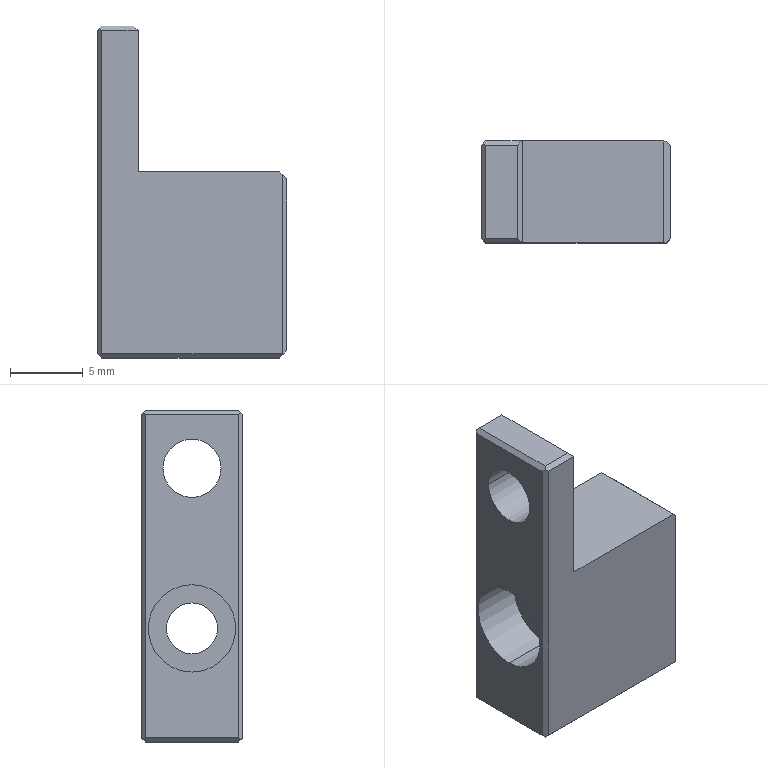Part | NX | 1 solid | 28 faces | box 13 x 7 x 22.8 mm | volume 1128 mm3 | plane 22 | cylinder 6 | commonest cylinder face diameters 3.5 x2 4 x2 6 x2
STEP:
#1=CARTESIAN_POINT('',(2192.3,158.2,-92.));
#2=VERTEX_POINT('',#1);
#3=CARTESIAN_POINT('',(2192.3,151.8,-92.));
#4=VERTEX_POINT('',#3);
#5=CARTESIAN_POINT('',(2192.3,155.,-92.));
#6=DIRECTION('',(0.,-1.,0.));
#7=VECTOR('',#6,1000.);
#8=LINE('',#5,#7);
#9=EDGE_CURVE('',#2,#4,#8,.T.);
#10=ORIENTED_EDGE('',*,*,#9,.T.);
#11=CARTESIAN_POINT('',(2194.5,151.8,-92.));
#12=VERTEX_POINT('',#11);
#13=CARTESIAN_POINT('',(2193.4,151.8,-92.));
#14=DIRECTION('',(-1.,0.,0.));
#15=VECTOR('',#14,1000.);
#16=LINE('',#13,#15);
#17=EDGE_CURVE('',#12,#4,#16,.T.);
#18=ORIENTED_EDGE('',*,*,#17,.F.);
#19=CARTESIAN_POINT('',(2194.5,158.2,-92.));
#20=VERTEX_POINT('',#19);
#21=CARTESIAN_POINT('',(2194.5,155.,-92.));
#22=DIRECTION('',(0.,1.,0.));
#23=VECTOR('',#22,1000.);
#24=LINE('',#21,#23);
#25=EDGE_CURVE('',#12,#20,#24,.T.);
#26=ORIENTED_EDGE('',*,*,#25,.T.);
#27=CARTESIAN_POINT('',(2193.4,158.2,-92.));
#28=DIRECTION('',(-1.,0.,0.));
#29=VECTOR('',#28,1000.);
#30=LINE('',#27,#29);
#31=EDGE_CURVE('',#20,#2,#30,.T.);
#32=ORIENTED_EDGE('',*,*,#31,.T.);
#33=EDGE_LOOP('',(#10,#18,#26,#32));
#34=FACE_BOUND('',#33,.T.);
#35=CARTESIAN_POINT('',(2192.,158.5,-92.));
#36=DIRECTION('',(0.,0.,1.));
#37=DIRECTION('',(1.,0.,0.));
#38=AXIS2_PLACEMENT_3D('',#35,#36,#37);
#39=PLANE('',#38);
#40=ADVANCED_FACE('',(#34),#39,.T.);
#41=CARTESIAN_POINT('',(2192.,158.2,-114.5));
#42=VERTEX_POINT('',#41);
#43=CARTESIAN_POINT('',(2192.,151.8,-114.5));
#44=VERTEX_POINT('',#43);
#45=CARTESIAN_POINT('',(2192.,155.,-114.5));
#46=DIRECTION('',(0.,-1.,0.));
#47=VECTOR('',#46,1000.);
#48=LINE('',#45,#47);
#49=EDGE_CURVE('',#42,#44,#48,.T.);
#50=ORIENTED_EDGE('',*,*,#49,.T.);
#51=CARTESIAN_POINT('',(2192.,151.8,-92.3));
#52=VERTEX_POINT('',#51);
#53=CARTESIAN_POINT('',(2192.,151.8,-102.539));
#54=DIRECTION('',(0.,0.,1.));
#55=VECTOR('',#54,1000.);
#56=LINE('',#53,#55);
#57=EDGE_CURVE('',#44,#52,#56,.T.);
#58=ORIENTED_EDGE('',*,*,#57,.T.);
#59=CARTESIAN_POINT('',(2192.,158.2,-92.3));
#60=VERTEX_POINT('',#59);
#61=CARTESIAN_POINT('',(2192.,155.,-92.3));
#62=DIRECTION('',(0.,-1.,0.));
#63=VECTOR('',#62,1000.);
#64=LINE('',#61,#63);
#65=EDGE_CURVE('',#60,#52,#64,.T.);
#66=ORIENTED_EDGE('',*,*,#65,.F.);
#67=CARTESIAN_POINT('',(2192.,158.2,-102.539));
#68=DIRECTION('',(0.,0.,1.));
#69=VECTOR('',#68,1000.);
#70=LINE('',#67,#69);
#71=EDGE_CURVE('',#42,#60,#70,.T.);
#72=ORIENTED_EDGE('',*,*,#71,.F.);
#73=EDGE_LOOP('',(#50,#58,#66,#72));
#74=FACE_BOUND('',#73,.T.);
#75=CARTESIAN_POINT('',(2192.,153.,-96.));
#76=VERTEX_POINT('',#75);
#77=CARTESIAN_POINT('',(2192.,157.,-96.));
#78=VERTEX_POINT('',#77);
#79=CARTESIAN_POINT('',(2192.,155.,-96.));
#80=DIRECTION('',(1.,0.,0.));
#81=DIRECTION('',(0.,1.,0.));
#82=AXIS2_PLACEMENT_3D('',#79,#80,#81);
#83=CIRCLE('',#82,2.);
#84=EDGE_CURVE('',#76,#78,#83,.T.);
#85=ORIENTED_EDGE('',*,*,#84,.T.);
#86=CARTESIAN_POINT('',(2192.,155.,-96.));
#87=DIRECTION('',(1.,0.,0.));
#88=DIRECTION('',(0.,1.,0.));
#89=AXIS2_PLACEMENT_3D('',#86,#87,#88);
#90=CIRCLE('',#89,2.);
#91=EDGE_CURVE('',#78,#76,#90,.T.);
#92=ORIENTED_EDGE('',*,*,#91,.T.);
#93=EDGE_LOOP('',(#85,#92));
#94=FACE_BOUND('',#93,.T.);
#95=CARTESIAN_POINT('',(2192.,155.,-110.));
#96=VERTEX_POINT('',#95);
#97=CARTESIAN_POINT('',(2192.,155.,-104.));
#98=VERTEX_POINT('',#97);
#99=CARTESIAN_POINT('',(2192.,155.,-107.));
#100=DIRECTION('',(-1.,0.,0.));
#101=DIRECTION('',(0.,0.,-1.));
#102=AXIS2_PLACEMENT_3D('',#99,#100,#101);
#103=CIRCLE('',#102,3.);
#104=EDGE_CURVE('',#96,#98,#103,.T.);
#105=ORIENTED_EDGE('',*,*,#104,.F.);
#106=CARTESIAN_POINT('',(2192.,155.,-107.));
#107=DIRECTION('',(-1.,0.,0.));
#108=DIRECTION('',(0.,0.,-1.));
#109=AXIS2_PLACEMENT_3D('',#106,#107,#108);
#110=CIRCLE('',#109,3.);
#111=EDGE_CURVE('',#98,#96,#110,.T.);
#112=ORIENTED_EDGE('',*,*,#111,.F.);
#113=EDGE_LOOP('',(#105,#112));
#114=FACE_BOUND('',#113,.T.);
#115=CARTESIAN_POINT('',(2192.,158.5,-112.));
#116=DIRECTION('',(-1.,0.,0.));
#117=DIRECTION('',(0.,0.,1.));
#118=AXIS2_PLACEMENT_3D('',#115,#116,#117);
#119=PLANE('',#118);
#120=ADVANCED_FACE('',(#74,#94,#114),#119,.T.);
#121=CARTESIAN_POINT('',(2204.5,151.8,-114.8));
#122=VERTEX_POINT('',#121);
#123=CARTESIAN_POINT('',(2204.5,158.2,-114.8));
#124=VERTEX_POINT('',#123);
#125=CARTESIAN_POINT('',(2204.5,155.,-114.8));
#126=DIRECTION('',(0.,1.,0.));
#127=VECTOR('',#126,1000.);
#128=LINE('',#125,#127);
#129=EDGE_CURVE('',#122,#124,#128,.T.);
#130=ORIENTED_EDGE('',*,*,#129,.F.);
#131=CARTESIAN_POINT('',(2192.3,151.8,-114.8));
#132=VERTEX_POINT('',#131);
#133=CARTESIAN_POINT('',(2198.5,151.8,-114.8));
#134=DIRECTION('',(-1.,0.,0.));
#135=VECTOR('',#134,1000.);
#136=LINE('',#133,#135);
#137=EDGE_CURVE('',#122,#132,#136,.T.);
#138=ORIENTED_EDGE('',*,*,#137,.T.);
#139=CARTESIAN_POINT('',(2192.3,158.2,-114.8));
#140=VERTEX_POINT('',#139);
#141=CARTESIAN_POINT('',(2192.3,155.,-114.8));
#142=DIRECTION('',(0.,-1.,0.));
#143=VECTOR('',#142,1000.);
#144=LINE('',#141,#143);
#145=EDGE_CURVE('',#140,#132,#144,.T.);
#146=ORIENTED_EDGE('',*,*,#145,.F.);
#147=CARTESIAN_POINT('',(2198.5,158.2,-114.8));
#148=DIRECTION('',(-1.,0.,0.));
#149=VECTOR('',#148,1000.);
#150=LINE('',#147,#149);
#151=EDGE_CURVE('',#124,#140,#150,.T.);
#152=ORIENTED_EDGE('',*,*,#151,.F.);
#153=EDGE_LOOP('',(#130,#138,#146,#152));
#154=FACE_BOUND('',#153,.T.);
#155=CARTESIAN_POINT('',(2200.,158.5,-114.8));
#156=DIRECTION('',(0.,0.,-1.));
#157=DIRECTION('',(0.,-1.,0.));
#158=AXIS2_PLACEMENT_3D('',#155,#156,#157);
#159=PLANE('',#158);
#160=ADVANCED_FACE('',(#154),#159,.T.);
#161=CARTESIAN_POINT('',(2205.,151.8,-114.3));
#162=VERTEX_POINT('',#161);
#163=CARTESIAN_POINT('',(2205.,158.2,-114.3));
#164=VERTEX_POINT('',#163);
#165=CARTESIAN_POINT('',(2205.,155.,-114.3));
#166=DIRECTION('',(0.,1.,0.));
#167=VECTOR('',#166,1000.);
#168=LINE('',#165,#167);
#169=EDGE_CURVE('',#162,#164,#168,.T.);
#170=ORIENTED_EDGE('',*,*,#169,.T.);
#171=CARTESIAN_POINT('',(2205.,158.2,-102.5));
#172=VERTEX_POINT('',#171);
#173=CARTESIAN_POINT('',(2205.,158.2,-102.539));
#174=DIRECTION('',(0.,0.,-1.));
#175=VECTOR('',#174,1000.);
#176=LINE('',#173,#175);
#177=EDGE_CURVE('',#172,#164,#176,.T.);
#178=ORIENTED_EDGE('',*,*,#177,.F.);
#179=CARTESIAN_POINT('',(2205.,151.8,-102.5));
#180=VERTEX_POINT('',#179);
#181=CARTESIAN_POINT('',(2205.,155.,-102.5));
#182=DIRECTION('',(0.,1.,0.));
#183=VECTOR('',#182,1000.);
#184=LINE('',#181,#183);
#185=EDGE_CURVE('',#180,#172,#184,.T.);
#186=ORIENTED_EDGE('',*,*,#185,.F.);
#187=CARTESIAN_POINT('',(2205.,151.8,-102.539));
#188=DIRECTION('',(0.,0.,-1.));
#189=VECTOR('',#188,1000.);
#190=LINE('',#187,#189);
#191=EDGE_CURVE('',#180,#162,#190,.T.);
#192=ORIENTED_EDGE('',*,*,#191,.T.);
#193=EDGE_LOOP('',(#170,#178,#186,#192));
#194=FACE_BOUND('',#193,.T.);
#195=CARTESIAN_POINT('',(2205.,155.,-105.25));
#196=VERTEX_POINT('',#195);
#197=CARTESIAN_POINT('',(2205.,155.,-108.75));
#198=VERTEX_POINT('',#197);
#199=CARTESIAN_POINT('',(2205.,155.,-107.));
#200=DIRECTION('',(-1.,0.,0.));
#201=DIRECTION('',(0.,0.,-1.));
#202=AXIS2_PLACEMENT_3D('',#199,#200,#201);
#203=CIRCLE('',#202,1.75);
#204=EDGE_CURVE('',#196,#198,#203,.T.);
#205=ORIENTED_EDGE('',*,*,#204,.T.);
#206=CARTESIAN_POINT('',(2205.,155.,-107.));
#207=DIRECTION('',(-1.,0.,0.));
#208=DIRECTION('',(0.,0.,-1.));
#209=AXIS2_PLACEMENT_3D('',#206,#207,#208);
#210=CIRCLE('',#209,1.75);
#211=EDGE_CURVE('',#198,#196,#210,.T.);
#212=ORIENTED_EDGE('',*,*,#211,.T.);
#213=EDGE_LOOP('',(#205,#212));
#214=FACE_BOUND('',#213,.T.);
#215=CARTESIAN_POINT('',(2205.,158.5,-102.));
#216=DIRECTION('',(1.,0.,0.));
#217=DIRECTION('',(0.,1.,0.));
#218=AXIS2_PLACEMENT_3D('',#215,#216,#217);
#219=PLANE('',#218);
#220=ADVANCED_FACE('',(#194,#214),#219,.T.);
#221=CARTESIAN_POINT('',(2194.8,158.5,-102.));
#222=VERTEX_POINT('',#221);
#223=CARTESIAN_POINT('',(2204.5,158.5,-102.));
#224=VERTEX_POINT('',#223);
#225=CARTESIAN_POINT('',(2208.515,158.5,-102.));
#226=DIRECTION('',(1.,0.,0.));
#227=VECTOR('',#226,1000.);
#228=LINE('',#225,#227);
#229=EDGE_CURVE('',#222,#224,#228,.T.);
#230=ORIENTED_EDGE('',*,*,#229,.F.);
#231=CARTESIAN_POINT('',(2194.8,151.5,-102.));
#232=VERTEX_POINT('',#231);
#233=CARTESIAN_POINT('',(2194.8,158.5,-102.));
#234=DIRECTION('',(0.,1.,0.));
#235=VECTOR('',#234,1000.);
#236=LINE('',#233,#235);
#237=EDGE_CURVE('',#232,#222,#236,.T.);
#238=ORIENTED_EDGE('',*,*,#237,.F.);
#239=CARTESIAN_POINT('',(2204.5,151.5,-102.));
#240=VERTEX_POINT('',#239);
#241=CARTESIAN_POINT('',(2208.515,151.5,-102.));
#242=DIRECTION('',(1.,0.,0.));
#243=VECTOR('',#242,1000.);
#244=LINE('',#241,#243);
#245=EDGE_CURVE('',#232,#240,#244,.T.);
#246=ORIENTED_EDGE('',*,*,#245,.T.);
#247=CARTESIAN_POINT('',(2204.5,155.,-102.));
#248=DIRECTION('',(0.,1.,0.));
#249=VECTOR('',#248,1000.);
#250=LINE('',#247,#249);
#251=EDGE_CURVE('',#240,#224,#250,.T.);
#252=ORIENTED_EDGE('',*,*,#251,.T.);
#253=EDGE_LOOP('',(#230,#238,#246,#252));
#254=FACE_BOUND('',#253,.T.);
#255=CARTESIAN_POINT('',(2195.,158.5,-102.));
#256=DIRECTION('',(0.,0.,1.));
#257=DIRECTION('',(1.,0.,0.));
#258=AXIS2_PLACEMENT_3D('',#255,#256,#257);
#259=PLANE('',#258);
#260=ADVANCED_FACE('',(#254),#259,.T.);
#261=CARTESIAN_POINT('',(2194.8,158.5,-92.3));
#262=VERTEX_POINT('',#261);
#263=CARTESIAN_POINT('',(2194.8,158.5,-102.539));
#264=DIRECTION('',(0.,0.,-1.));
#265=VECTOR('',#264,1000.);
#266=LINE('',#263,#265);
#267=EDGE_CURVE('',#262,#222,#266,.T.);
#268=ORIENTED_EDGE('',*,*,#267,.F.);
#269=CARTESIAN_POINT('',(2194.8,151.5,-92.3));
#270=VERTEX_POINT('',#269);
#271=CARTESIAN_POINT('',(2194.8,155.,-92.3));
#272=DIRECTION('',(0.,1.,0.));
#273=VECTOR('',#272,1000.);
#274=LINE('',#271,#273);
#275=EDGE_CURVE('',#270,#262,#274,.T.);
#276=ORIENTED_EDGE('',*,*,#275,.F.);
#277=CARTESIAN_POINT('',(2194.8,151.5,-102.539));
#278=DIRECTION('',(0.,0.,-1.));
#279=VECTOR('',#278,1000.);
#280=LINE('',#277,#279);
#281=EDGE_CURVE('',#270,#232,#280,.T.);
#282=ORIENTED_EDGE('',*,*,#281,.T.);
#283=ORIENTED_EDGE('',*,*,#237,.T.);
#284=EDGE_LOOP('',(#268,#276,#282,#283));
#285=FACE_BOUND('',#284,.T.);
#286=CARTESIAN_POINT('',(2194.8,153.,-96.));
#287=VERTEX_POINT('',#286);
#288=CARTESIAN_POINT('',(2194.8,157.,-96.));
#289=VERTEX_POINT('',#288);
#290=CARTESIAN_POINT('',(2194.8,155.,-96.));
#291=DIRECTION('',(1.,0.,0.));
#292=DIRECTION('',(0.,1.,0.));
#293=AXIS2_PLACEMENT_3D('',#290,#291,#292);
#294=CIRCLE('',#293,2.);
#295=EDGE_CURVE('',#287,#289,#294,.T.);
#296=ORIENTED_EDGE('',*,*,#295,.F.);
#297=CARTESIAN_POINT('',(2194.8,155.,-96.));
#298=DIRECTION('',(1.,0.,0.));
#299=DIRECTION('',(0.,1.,0.));
#300=AXIS2_PLACEMENT_3D('',#297,#298,#299);
#301=CIRCLE('',#300,2.);
#302=EDGE_CURVE('',#289,#287,#301,.T.);
#303=ORIENTED_EDGE('',*,*,#302,.F.);
#304=EDGE_LOOP('',(#296,#303));
#305=FACE_BOUND('',#304,.T.);
#306=CARTESIAN_POINT('',(2194.8,158.5,-92.));
#307=DIRECTION('',(1.,0.,0.));
#308=DIRECTION('',(0.,1.,0.));
#309=AXIS2_PLACEMENT_3D('',#306,#307,#308);
#310=PLANE('',#309);
#311=ADVANCED_FACE('',(#285,#305),#310,.T.);
#312=CARTESIAN_POINT('',(2195.5,155.,-110.));
#313=VERTEX_POINT('',#312);
#314=CARTESIAN_POINT('',(2195.5,155.,-104.));
#315=VERTEX_POINT('',#314);
#316=CARTESIAN_POINT('',(2195.5,155.,-107.));
#317=DIRECTION('',(-1.,0.,0.));
#318=DIRECTION('',(0.,0.,-1.));
#319=AXIS2_PLACEMENT_3D('',#316,#317,#318);
#320=CIRCLE('',#319,3.);
#321=EDGE_CURVE('',#313,#315,#320,.T.);
#322=ORIENTED_EDGE('',*,*,#321,.F.);
#323=CARTESIAN_POINT('',(2192.,155.,-110.));
#324=DIRECTION('',(-1.,0.,0.));
#325=VECTOR('',#324,1000.);
#326=LINE('',#323,#325);
#327=EDGE_CURVE('',#96,#313,#326,.F.);
#328=ORIENTED_EDGE('',*,*,#327,.F.);
#329=ORIENTED_EDGE('',*,*,#104,.T.);
#330=CARTESIAN_POINT('',(2192.,155.,-104.));
#331=DIRECTION('',(-1.,0.,0.));
#332=VECTOR('',#331,1000.);
#333=LINE('',#330,#332);
#334=EDGE_CURVE('',#98,#315,#333,.F.);
#335=ORIENTED_EDGE('',*,*,#334,.T.);
#336=EDGE_LOOP('',(#322,#328,#329,#335));
#337=FACE_BOUND('',#336,.T.);
#338=CARTESIAN_POINT('',(2192.,155.,-107.));
#339=DIRECTION('',(-1.,0.,0.));
#340=DIRECTION('',(0.,0.,-1.));
#341=AXIS2_PLACEMENT_3D('',#338,#339,#340);
#342=CYLINDRICAL_SURFACE('',#341,3.);
#343=ADVANCED_FACE('',(#337),#342,.F.);
#344=ORIENTED_EDGE('',*,*,#321,.T.);
#345=CARTESIAN_POINT('',(2195.5,155.,-107.));
#346=DIRECTION('',(-1.,0.,0.));
#347=DIRECTION('',(0.,0.,-1.));
#348=AXIS2_PLACEMENT_3D('',#345,#346,#347);
#349=CIRCLE('',#348,3.);
#350=EDGE_CURVE('',#315,#313,#349,.T.);
#351=ORIENTED_EDGE('',*,*,#350,.T.);
#352=EDGE_LOOP('',(#344,#351));
#353=FACE_BOUND('',#352,.T.);
#354=CARTESIAN_POINT('',(2195.5,155.,-105.25));
#355=VERTEX_POINT('',#354);
#356=CARTESIAN_POINT('',(2195.5,155.,-108.75));
#357=VERTEX_POINT('',#356);
#358=CARTESIAN_POINT('',(2195.5,155.,-107.));
#359=DIRECTION('',(-1.,0.,0.));
#360=DIRECTION('',(0.,0.,-1.));
#361=AXIS2_PLACEMENT_3D('',#358,#359,#360);
#362=CIRCLE('',#361,1.75);
#363=EDGE_CURVE('',#355,#357,#362,.T.);
#364=ORIENTED_EDGE('',*,*,#363,.F.);
#365=CARTESIAN_POINT('',(2195.5,155.,-107.));
#366=DIRECTION('',(-1.,0.,0.));
#367=DIRECTION('',(0.,0.,-1.));
#368=AXIS2_PLACEMENT_3D('',#365,#366,#367);
#369=CIRCLE('',#368,1.75);
#370=EDGE_CURVE('',#357,#355,#369,.T.);
#371=ORIENTED_EDGE('',*,*,#370,.F.);
#372=EDGE_LOOP('',(#364,#371));
#373=FACE_BOUND('',#372,.T.);
#374=CARTESIAN_POINT('',(2195.5,155.,-107.));
#375=DIRECTION('',(-1.,0.,0.));
#376=DIRECTION('',(0.,0.,1.));
#377=AXIS2_PLACEMENT_3D('',#374,#375,#376);
#378=PLANE('',#377);
#379=ADVANCED_FACE('',(#353,#373),#378,.T.);
#380=ORIENTED_EDGE('',*,*,#204,.F.);
#381=CARTESIAN_POINT('',(2192.,155.,-105.25));
#382=DIRECTION('',(-1.,0.,0.));
#383=VECTOR('',#382,1000.);
#384=LINE('',#381,#383);
#385=EDGE_CURVE('',#355,#196,#384,.F.);
#386=ORIENTED_EDGE('',*,*,#385,.F.);
#387=ORIENTED_EDGE('',*,*,#363,.T.);
#388=CARTESIAN_POINT('',(2192.,155.,-108.75));
#389=DIRECTION('',(-1.,0.,0.));
#390=VECTOR('',#389,1000.);
#391=LINE('',#388,#390);
#392=EDGE_CURVE('',#357,#198,#391,.F.);
#393=ORIENTED_EDGE('',*,*,#392,.T.);
#394=EDGE_LOOP('',(#380,#386,#387,#393));
#395=FACE_BOUND('',#394,.T.);
#396=CARTESIAN_POINT('',(2192.,155.,-107.));
#397=DIRECTION('',(-1.,0.,0.));
#398=DIRECTION('',(0.,0.,-1.));
#399=AXIS2_PLACEMENT_3D('',#396,#397,#398);
#400=CYLINDRICAL_SURFACE('',#399,1.75);
#401=ADVANCED_FACE('',(#395),#400,.F.);
#402=ORIENTED_EDGE('',*,*,#9,.F.);
#403=CARTESIAN_POINT('',(2192.15,158.35,-92.15));
#404=VERTEX_POINT('',#403);
#405=CARTESIAN_POINT('',(2181.761,168.739,-102.539));
#406=DIRECTION('',(-0.5774,0.5774,-0.5774));
#407=VECTOR('',#406,1000.);
#408=LINE('',#405,#407);
#409=EDGE_CURVE('',#2,#404,#408,.T.);
#410=ORIENTED_EDGE('',*,*,#409,.T.);
#411=CARTESIAN_POINT('',(2181.761,147.961,-102.539));
#412=DIRECTION('',(-0.5774,-0.5774,-0.5774));
#413=VECTOR('',#412,1000.);
#414=LINE('',#411,#413);
#415=EDGE_CURVE('',#404,#60,#414,.T.);
#416=ORIENTED_EDGE('',*,*,#415,.T.);
#417=ORIENTED_EDGE('',*,*,#65,.T.);
#418=CARTESIAN_POINT('',(2192.15,151.65,-92.15));
#419=VERTEX_POINT('',#418);
#420=CARTESIAN_POINT('',(2181.761,162.039,-102.539));
#421=DIRECTION('',(-0.5774,0.5774,-0.5774));
#422=VECTOR('',#421,1000.);
#423=LINE('',#420,#422);
#424=EDGE_CURVE('',#419,#52,#423,.T.);
#425=ORIENTED_EDGE('',*,*,#424,.F.);
#426=CARTESIAN_POINT('',(2181.761,141.261,-102.539));
#427=DIRECTION('',(-0.5774,-0.5774,-0.5774));
#428=VECTOR('',#427,1000.);
#429=LINE('',#426,#428);
#430=EDGE_CURVE('',#4,#419,#429,.T.);
#431=ORIENTED_EDGE('',*,*,#430,.F.);
#432=EDGE_LOOP('',(#402,#410,#416,#417,#425,#431));
#433=FACE_BOUND('',#432,.T.);
#434=CARTESIAN_POINT('',(2192.15,155.,-92.15));
#435=DIRECTION('',(-0.7071,0.,0.7071));
#436=DIRECTION('',(0.,1.,0.));
#437=AXIS2_PLACEMENT_3D('',#434,#435,#436);
#438=PLANE('',#437);
#439=ADVANCED_FACE('',(#433),#438,.T.);
#440=ORIENTED_EDGE('',*,*,#185,.T.);
#441=CARTESIAN_POINT('',(2204.7,158.5,-102.2));
#442=VERTEX_POINT('',#441);
#443=CARTESIAN_POINT('',(2204.7,158.5,-102.2));
#444=DIRECTION('',(0.5774,-0.5774,-0.5774));
#445=VECTOR('',#444,1000.);
#446=LINE('',#443,#445);
#447=EDGE_CURVE('',#442,#172,#446,.T.);
#448=ORIENTED_EDGE('',*,*,#447,.F.);
#449=CARTESIAN_POINT('',(2205.039,158.5,-102.539));
#450=DIRECTION('',(0.7071,0.,-0.7071));
#451=VECTOR('',#450,1000.);
#452=LINE('',#449,#451);
#453=EDGE_CURVE('',#224,#442,#452,.T.);
#454=ORIENTED_EDGE('',*,*,#453,.F.);
#455=ORIENTED_EDGE('',*,*,#251,.F.);
#456=CARTESIAN_POINT('',(2204.7,151.5,-102.2));
#457=VERTEX_POINT('',#456);
#458=CARTESIAN_POINT('',(2205.039,151.5,-102.539));
#459=DIRECTION('',(0.7071,0.,-0.7071));
#460=VECTOR('',#459,1000.);
#461=LINE('',#458,#460);
#462=EDGE_CURVE('',#240,#457,#461,.T.);
#463=ORIENTED_EDGE('',*,*,#462,.T.);
#464=CARTESIAN_POINT('',(2211.7,158.5,-109.2));
#465=DIRECTION('',(0.5774,0.5774,-0.5774));
#466=VECTOR('',#465,1000.);
#467=LINE('',#464,#466);
#468=EDGE_CURVE('',#457,#180,#467,.T.);
#469=ORIENTED_EDGE('',*,*,#468,.T.);
#470=EDGE_LOOP('',(#440,#448,#454,#455,#463,#469));
#471=FACE_BOUND('',#470,.T.);
#472=CARTESIAN_POINT('',(2204.75,155.,-102.25));
#473=DIRECTION('',(-0.7071,0.,-0.7071));
#474=DIRECTION('',(-0.7071,0.,0.7071));
#475=AXIS2_PLACEMENT_3D('',#472,#473,#474);
#476=PLANE('',#475);
#477=ADVANCED_FACE('',(#471),#476,.F.);
#478=ORIENTED_EDGE('',*,*,#84,.F.);
#479=CARTESIAN_POINT('',(2200.8,153.,-96.));
#480=DIRECTION('',(1.,0.,0.));
#481=VECTOR('',#480,1000.);
#482=LINE('',#479,#481);
#483=EDGE_CURVE('',#76,#287,#482,.T.);
#484=ORIENTED_EDGE('',*,*,#483,.T.);
#485=ORIENTED_EDGE('',*,*,#295,.T.);
#486=CARTESIAN_POINT('',(2200.8,157.,-96.));
#487=DIRECTION('',(1.,0.,0.));
#488=VECTOR('',#487,1000.);
#489=LINE('',#486,#488);
#490=EDGE_CURVE('',#78,#289,#489,.T.);
#491=ORIENTED_EDGE('',*,*,#490,.F.);
#492=EDGE_LOOP('',(#478,#484,#485,#491));
#493=FACE_BOUND('',#492,.T.);
#494=CARTESIAN_POINT('',(2200.8,155.,-96.));
#495=DIRECTION('',(1.,0.,0.));
#496=DIRECTION('',(0.,1.,0.));
#497=AXIS2_PLACEMENT_3D('',#494,#495,#496);
#498=CYLINDRICAL_SURFACE('',#497,2.);
#499=ADVANCED_FACE('',(#493),#498,.F.);
#500=ORIENTED_EDGE('',*,*,#25,.F.);
#501=CARTESIAN_POINT('',(2205.039,141.261,-102.539));
#502=DIRECTION('',(0.5774,-0.5774,-0.5774));
#503=VECTOR('',#502,1000.);
#504=LINE('',#501,#503);
#505=EDGE_CURVE('',#12,#270,#504,.T.);
#506=ORIENTED_EDGE('',*,*,#505,.T.);
#507=ORIENTED_EDGE('',*,*,#275,.T.);
#508=CARTESIAN_POINT('',(2205.039,168.739,-102.539));
#509=DIRECTION('',(-0.5774,-0.5774,0.5774));
#510=VECTOR('',#509,1000.);
#511=LINE('',#508,#510);
#512=EDGE_CURVE('',#262,#20,#511,.T.);
#513=ORIENTED_EDGE('',*,*,#512,.T.);
#514=EDGE_LOOP('',(#500,#506,#507,#513));
#515=FACE_BOUND('',#514,.T.);
#516=CARTESIAN_POINT('',(2194.65,155.,-92.15));
#517=DIRECTION('',(0.7071,0.,0.7071));
#518=DIRECTION('',(0.,-1.,0.));
#519=AXIS2_PLACEMENT_3D('',#516,#517,#518);
#520=PLANE('',#519);
#521=ADVANCED_FACE('',(#515),#520,.T.);
#522=ORIENTED_EDGE('',*,*,#129,.T.);
#523=CARTESIAN_POINT('',(2204.75,158.45,-114.55));
#524=VERTEX_POINT('',#523);
#525=CARTESIAN_POINT('',(2216.761,170.461,-102.539));
#526=DIRECTION('',(-0.5774,-0.5774,-0.5774));
#527=VECTOR('',#526,1000.);
#528=LINE('',#525,#527);
#529=EDGE_CURVE('',#524,#124,#528,.T.);
#530=ORIENTED_EDGE('',*,*,#529,.F.);
#531=CARTESIAN_POINT('',(2204.7,158.5,-114.6));
#532=DIRECTION('',(-0.5774,0.5774,-0.5774));
#533=VECTOR('',#532,1000.);
#534=LINE('',#531,#533);
#535=EDGE_CURVE('',#164,#524,#534,.T.);
#536=ORIENTED_EDGE('',*,*,#535,.F.);
#537=ORIENTED_EDGE('',*,*,#169,.F.);
#538=CARTESIAN_POINT('',(2204.75,151.55,-114.55));
#539=VERTEX_POINT('',#538);
#540=CARTESIAN_POINT('',(2211.7,158.5,-107.6));
#541=DIRECTION('',(-0.5774,-0.5774,-0.5774));
#542=VECTOR('',#541,1000.);
#543=LINE('',#540,#542);
#544=EDGE_CURVE('',#162,#539,#543,.T.);
#545=ORIENTED_EDGE('',*,*,#544,.T.);
#546=CARTESIAN_POINT('',(2216.761,139.539,-102.539));
#547=DIRECTION('',(-0.5774,0.5774,-0.5774));
#548=VECTOR('',#547,1000.);
#549=LINE('',#546,#548);
#550=EDGE_CURVE('',#539,#122,#549,.T.);
#551=ORIENTED_EDGE('',*,*,#550,.T.);
#552=EDGE_LOOP('',(#522,#530,#536,#537,#545,#551));
#553=FACE_BOUND('',#552,.T.);
#554=CARTESIAN_POINT('',(2204.75,155.,-114.55));
#555=DIRECTION('',(-0.7071,0.,0.7071));
#556=DIRECTION('',(0.,1.,0.));
#557=AXIS2_PLACEMENT_3D('',#554,#555,#556);
#558=PLANE('',#557);
#559=ADVANCED_FACE('',(#553),#558,.F.);
#560=ORIENTED_EDGE('',*,*,#49,.F.);
#561=CARTESIAN_POINT('',(2192.15,158.35,-114.65));
#562=VERTEX_POINT('',#561);
#563=CARTESIAN_POINT('',(2180.039,146.239,-102.539));
#564=DIRECTION('',(0.5774,0.5774,-0.5774));
#565=VECTOR('',#564,1000.);
#566=LINE('',#563,#565);
#567=EDGE_CURVE('',#42,#562,#566,.T.);
#568=ORIENTED_EDGE('',*,*,#567,.T.);
#569=CARTESIAN_POINT('',(2180.039,170.461,-102.539));
#570=DIRECTION('',(0.5774,-0.5774,-0.5774));
#571=VECTOR('',#570,1000.);
#572=LINE('',#569,#571);
#573=EDGE_CURVE('',#562,#140,#572,.T.);
#574=ORIENTED_EDGE('',*,*,#573,.T.);
#575=ORIENTED_EDGE('',*,*,#145,.T.);
#576=CARTESIAN_POINT('',(2192.15,151.65,-114.65));
#577=VERTEX_POINT('',#576);
#578=CARTESIAN_POINT('',(2180.039,139.539,-102.539));
#579=DIRECTION('',(-0.5774,-0.5774,0.5774));
#580=VECTOR('',#579,1000.);
#581=LINE('',#578,#580);
#582=EDGE_CURVE('',#132,#577,#581,.T.);
#583=ORIENTED_EDGE('',*,*,#582,.T.);
#584=CARTESIAN_POINT('',(2180.039,163.761,-102.539));
#585=DIRECTION('',(0.5774,-0.5774,-0.5774));
#586=VECTOR('',#585,1000.);
#587=LINE('',#584,#586);
#588=EDGE_CURVE('',#44,#577,#587,.T.);
#589=ORIENTED_EDGE('',*,*,#588,.F.);
#590=EDGE_LOOP('',(#560,#568,#574,#575,#583,#589));
#591=FACE_BOUND('',#590,.T.);
#592=CARTESIAN_POINT('',(2192.15,155.,-114.65));
#593=DIRECTION('',(-0.7071,0.,-0.7071));
#594=DIRECTION('',(-0.7071,0.,0.7071));
#595=AXIS2_PLACEMENT_3D('',#592,#593,#594);
#596=PLANE('',#595);
#597=ADVANCED_FACE('',(#591),#596,.T.);
#598=CARTESIAN_POINT('',(2192.3,158.5,-114.5));
#599=VERTEX_POINT('',#598);
#600=CARTESIAN_POINT('',(2192.3,158.5,-92.3));
#601=VERTEX_POINT('',#600);
#602=CARTESIAN_POINT('',(2192.3,158.5,-102.539));
#603=DIRECTION('',(0.,0.,1.));
#604=VECTOR('',#603,1000.);
#605=LINE('',#602,#604);
#606=EDGE_CURVE('',#599,#601,#605,.T.);
#607=ORIENTED_EDGE('',*,*,#606,.F.);
#608=CARTESIAN_POINT('',(2204.261,170.461,-102.539));
#609=DIRECTION('',(0.5774,0.5774,0.5774));
#610=VECTOR('',#609,1000.);
#611=LINE('',#608,#610);
#612=EDGE_CURVE('',#562,#599,#611,.T.);
#613=ORIENTED_EDGE('',*,*,#612,.F.);
#614=ORIENTED_EDGE('',*,*,#567,.F.);
#615=ORIENTED_EDGE('',*,*,#71,.T.);
#616=ORIENTED_EDGE('',*,*,#415,.F.);
#617=CARTESIAN_POINT('',(2202.539,168.739,-102.539));
#618=DIRECTION('',(0.5774,0.5774,-0.5774));
#619=VECTOR('',#618,1000.);
#620=LINE('',#617,#619);
#621=EDGE_CURVE('',#404,#601,#620,.T.);
#622=ORIENTED_EDGE('',*,*,#621,.T.);
#623=EDGE_LOOP('',(#607,#613,#614,#615,#616,#622));
#624=FACE_BOUND('',#623,.T.);
#625=CARTESIAN_POINT('',(2192.15,158.35,-101.9));
#626=DIRECTION('',(-0.7071,0.7071,0.));
#627=DIRECTION('',(0.,0.,1.));
#628=AXIS2_PLACEMENT_3D('',#625,#626,#627);
#629=PLANE('',#628);
#630=ADVANCED_FACE('',(#624),#629,.T.);
#631=ORIENTED_EDGE('',*,*,#177,.T.);
#632=ORIENTED_EDGE('',*,*,#535,.T.);
#633=CARTESIAN_POINT('',(2204.7,158.5,-114.5));
#634=VERTEX_POINT('',#633);
#635=CARTESIAN_POINT('',(2192.739,170.461,-102.539));
#636=DIRECTION('',(0.5774,-0.5774,-0.5774));
#637=VECTOR('',#636,1000.);
#638=LINE('',#635,#637);
#639=EDGE_CURVE('',#634,#524,#638,.T.);
#640=ORIENTED_EDGE('',*,*,#639,.F.);
#641=CARTESIAN_POINT('',(2204.7,158.5,-102.539));
#642=DIRECTION('',(0.,0.,-1.));
#643=VECTOR('',#642,1000.);
#644=LINE('',#641,#643);
#645=EDGE_CURVE('',#442,#634,#644,.T.);
#646=ORIENTED_EDGE('',*,*,#645,.F.);
#647=ORIENTED_EDGE('',*,*,#447,.T.);
#648=EDGE_LOOP('',(#631,#632,#640,#646,#647));
#649=FACE_BOUND('',#648,.T.);
#650=CARTESIAN_POINT('',(2204.85,158.35,-106.75));
#651=DIRECTION('',(0.7071,0.7071,0.));
#652=DIRECTION('',(0.,0.,-1.));
#653=AXIS2_PLACEMENT_3D('',#650,#651,#652);
#654=PLANE('',#653);
#655=ADVANCED_FACE('',(#649),#654,.T.);
#656=CARTESIAN_POINT('',(2198.5,158.5,-114.5));
#657=DIRECTION('',(-1.,0.,0.));
#658=VECTOR('',#657,1000.);
#659=LINE('',#656,#658);
#660=EDGE_CURVE('',#634,#599,#659,.T.);
#661=ORIENTED_EDGE('',*,*,#660,.F.);
#662=ORIENTED_EDGE('',*,*,#639,.T.);
#663=ORIENTED_EDGE('',*,*,#529,.T.);
#664=ORIENTED_EDGE('',*,*,#151,.T.);
#665=ORIENTED_EDGE('',*,*,#573,.F.);
#666=ORIENTED_EDGE('',*,*,#612,.T.);
#667=EDGE_LOOP('',(#661,#662,#663,#664,#665,#666));
#668=FACE_BOUND('',#667,.T.);
#669=CARTESIAN_POINT('',(2198.5,158.35,-114.65));
#670=DIRECTION('',(0.,0.7071,-0.7071));
#671=DIRECTION('',(-1.,0.,0.));
#672=AXIS2_PLACEMENT_3D('',#669,#670,#671);
#673=PLANE('',#672);
#674=ADVANCED_FACE('',(#668),#673,.T.);
#675=CARTESIAN_POINT('',(2204.7,151.5,-114.5));
#676=VERTEX_POINT('',#675);
#677=CARTESIAN_POINT('',(2192.3,151.5,-114.5));
#678=VERTEX_POINT('',#677);
#679=CARTESIAN_POINT('',(2198.5,151.5,-114.5));
#680=DIRECTION('',(-1.,0.,0.));
#681=VECTOR('',#680,1000.);
#682=LINE('',#679,#681);
#683=EDGE_CURVE('',#676,#678,#682,.T.);
#684=ORIENTED_EDGE('',*,*,#683,.F.);
#685=CARTESIAN_POINT('',(2204.7,151.5,-102.539));
#686=DIRECTION('',(0.,0.,-1.));
#687=VECTOR('',#686,1000.);
#688=LINE('',#685,#687);
#689=EDGE_CURVE('',#457,#676,#688,.T.);
#690=ORIENTED_EDGE('',*,*,#689,.F.);
#691=ORIENTED_EDGE('',*,*,#462,.F.);
#692=ORIENTED_EDGE('',*,*,#245,.F.);
#693=ORIENTED_EDGE('',*,*,#281,.F.);
#694=CARTESIAN_POINT('',(2192.3,151.5,-92.3));
#695=VERTEX_POINT('',#694);
#696=CARTESIAN_POINT('',(2193.4,151.5,-92.3));
#697=DIRECTION('',(-1.,0.,0.));
#698=VECTOR('',#697,1000.);
#699=LINE('',#696,#698);
#700=EDGE_CURVE('',#270,#695,#699,.T.);
#701=ORIENTED_EDGE('',*,*,#700,.T.);
#702=CARTESIAN_POINT('',(2192.3,151.5,-102.539));
#703=DIRECTION('',(0.,0.,1.));
#704=VECTOR('',#703,1000.);
#705=LINE('',#702,#704);
#706=EDGE_CURVE('',#678,#695,#705,.T.);
#707=ORIENTED_EDGE('',*,*,#706,.F.);
#708=EDGE_LOOP('',(#684,#690,#691,#692,#693,#701,#707));
#709=FACE_BOUND('',#708,.T.);
#710=CARTESIAN_POINT('',(2208.515,151.5,-102.539));
#711=DIRECTION('',(0.,1.,0.));
#712=DIRECTION('',(1.,0.,0.));
#713=AXIS2_PLACEMENT_3D('',#710,#711,#712);
#714=PLANE('',#713);
#715=ADVANCED_FACE('',(#709),#714,.F.);
#716=ORIENTED_EDGE('',*,*,#700,.F.);
#717=ORIENTED_EDGE('',*,*,#505,.F.);
#718=ORIENTED_EDGE('',*,*,#17,.T.);
#719=ORIENTED_EDGE('',*,*,#430,.T.);
#720=CARTESIAN_POINT('',(2202.539,141.261,-102.539));
#721=DIRECTION('',(-0.5774,0.5774,0.5774));
#722=VECTOR('',#721,1000.);
#723=LINE('',#720,#722);
#724=EDGE_CURVE('',#695,#419,#723,.T.);
#725=ORIENTED_EDGE('',*,*,#724,.F.);
#726=EDGE_LOOP('',(#716,#717,#718,#719,#725));
#727=FACE_BOUND('',#726,.T.);
#728=CARTESIAN_POINT('',(2193.4,151.65,-92.15));
#729=DIRECTION('',(0.,-0.7071,0.7071));
#730=DIRECTION('',(-1.,0.,0.));
#731=AXIS2_PLACEMENT_3D('',#728,#729,#730);
#732=PLANE('',#731);
#733=ADVANCED_FACE('',(#727),#732,.T.);
#734=ORIENTED_EDGE('',*,*,#57,.F.);
#735=ORIENTED_EDGE('',*,*,#588,.T.);
#736=CARTESIAN_POINT('',(2204.261,139.539,-102.539));
#737=DIRECTION('',(-0.5774,0.5774,-0.5774));
#738=VECTOR('',#737,1000.);
#739=LINE('',#736,#738);
#740=EDGE_CURVE('',#678,#577,#739,.T.);
#741=ORIENTED_EDGE('',*,*,#740,.F.);
#742=ORIENTED_EDGE('',*,*,#706,.T.);
#743=ORIENTED_EDGE('',*,*,#724,.T.);
#744=ORIENTED_EDGE('',*,*,#424,.T.);
#745=EDGE_LOOP('',(#734,#735,#741,#742,#743,#744));
#746=FACE_BOUND('',#745,.T.);
#747=CARTESIAN_POINT('',(2192.15,151.65,-101.9));
#748=DIRECTION('',(0.7071,0.7071,0.));
#749=DIRECTION('',(0.,0.,-1.));
#750=AXIS2_PLACEMENT_3D('',#747,#748,#749);
#751=PLANE('',#750);
#752=ADVANCED_FACE('',(#746),#751,.F.);
#753=ORIENTED_EDGE('',*,*,#689,.T.);
#754=CARTESIAN_POINT('',(2192.739,139.539,-102.539));
#755=DIRECTION('',(-0.5774,-0.5774,0.5774));
#756=VECTOR('',#755,1000.);
#757=LINE('',#754,#756);
#758=EDGE_CURVE('',#539,#676,#757,.T.);
#759=ORIENTED_EDGE('',*,*,#758,.F.);
#760=ORIENTED_EDGE('',*,*,#544,.F.);
#761=ORIENTED_EDGE('',*,*,#191,.F.);
#762=ORIENTED_EDGE('',*,*,#468,.F.);
#763=EDGE_LOOP('',(#753,#759,#760,#761,#762));
#764=FACE_BOUND('',#763,.T.);
#765=CARTESIAN_POINT('',(2204.85,151.65,-106.75));
#766=DIRECTION('',(-0.7071,0.7071,0.));
#767=DIRECTION('',(0.,0.,1.));
#768=AXIS2_PLACEMENT_3D('',#765,#766,#767);
#769=PLANE('',#768);
#770=ADVANCED_FACE('',(#764),#769,.F.);
#771=ORIENTED_EDGE('',*,*,#683,.T.);
#772=ORIENTED_EDGE('',*,*,#740,.T.);
#773=ORIENTED_EDGE('',*,*,#582,.F.);
#774=ORIENTED_EDGE('',*,*,#137,.F.);
#775=ORIENTED_EDGE('',*,*,#550,.F.);
#776=ORIENTED_EDGE('',*,*,#758,.T.);
#777=EDGE_LOOP('',(#771,#772,#773,#774,#775,#776));
#778=FACE_BOUND('',#777,.T.);
#779=CARTESIAN_POINT('',(2198.5,151.65,-114.65));
#780=DIRECTION('',(0.,0.7071,0.7071));
#781=DIRECTION('',(1.,0.,0.));
#782=AXIS2_PLACEMENT_3D('',#779,#780,#781);
#783=PLANE('',#782);
#784=ADVANCED_FACE('',(#778),#783,.F.);
#785=ORIENTED_EDGE('',*,*,#660,.T.);
#786=ORIENTED_EDGE('',*,*,#606,.T.);
#787=CARTESIAN_POINT('',(2193.4,158.5,-92.3));
#788=DIRECTION('',(-1.,0.,0.));
#789=VECTOR('',#788,1000.);
#790=LINE('',#787,#789);
#791=EDGE_CURVE('',#262,#601,#790,.T.);
#792=ORIENTED_EDGE('',*,*,#791,.F.);
#793=ORIENTED_EDGE('',*,*,#267,.T.);
#794=ORIENTED_EDGE('',*,*,#229,.T.);
#795=ORIENTED_EDGE('',*,*,#453,.T.);
#796=ORIENTED_EDGE('',*,*,#645,.T.);
#797=EDGE_LOOP('',(#785,#786,#792,#793,#794,#795,#796));
#798=FACE_BOUND('',#797,.T.);
#799=CARTESIAN_POINT('',(2208.515,158.5,-102.539));
#800=DIRECTION('',(0.,1.,0.));
#801=DIRECTION('',(1.,0.,0.));
#802=AXIS2_PLACEMENT_3D('',#799,#800,#801);
#803=PLANE('',#802);
#804=ADVANCED_FACE('',(#798),#803,.T.);
#805=ORIENTED_EDGE('',*,*,#791,.T.);
#806=ORIENTED_EDGE('',*,*,#621,.F.);
#807=ORIENTED_EDGE('',*,*,#409,.F.);
#808=ORIENTED_EDGE('',*,*,#31,.F.);
#809=ORIENTED_EDGE('',*,*,#512,.F.);
#810=EDGE_LOOP('',(#805,#806,#807,#808,#809));
#811=FACE_BOUND('',#810,.T.);
#812=CARTESIAN_POINT('',(2193.4,158.35,-92.15));
#813=DIRECTION('',(0.,-0.7071,-0.7071));
#814=DIRECTION('',(0.,0.7071,-0.7071));
#815=AXIS2_PLACEMENT_3D('',#812,#813,#814);
#816=PLANE('',#815);
#817=ADVANCED_FACE('',(#811),#816,.F.);
#818=ORIENTED_EDGE('',*,*,#392,.F.);
#819=ORIENTED_EDGE('',*,*,#370,.T.);
#820=ORIENTED_EDGE('',*,*,#385,.T.);
#821=ORIENTED_EDGE('',*,*,#211,.F.);
#822=EDGE_LOOP('',(#818,#819,#820,#821));
#823=FACE_BOUND('',#822,.T.);
#824=CARTESIAN_POINT('',(2192.,155.,-107.));
#825=DIRECTION('',(-1.,0.,0.));
#826=DIRECTION('',(0.,0.,-1.));
#827=AXIS2_PLACEMENT_3D('',#824,#825,#826);
#828=CYLINDRICAL_SURFACE('',#827,1.75);
#829=ADVANCED_FACE('',(#823),#828,.F.);
#830=ORIENTED_EDGE('',*,*,#327,.T.);
#831=ORIENTED_EDGE('',*,*,#350,.F.);
#832=ORIENTED_EDGE('',*,*,#334,.F.);
#833=ORIENTED_EDGE('',*,*,#111,.T.);
#834=EDGE_LOOP('',(#830,#831,#832,#833));
#835=FACE_BOUND('',#834,.T.);
#836=CARTESIAN_POINT('',(2192.,155.,-107.));
#837=DIRECTION('',(-1.,0.,0.));
#838=DIRECTION('',(0.,0.,-1.));
#839=AXIS2_PLACEMENT_3D('',#836,#837,#838);
#840=CYLINDRICAL_SURFACE('',#839,3.);
#841=ADVANCED_FACE('',(#835),#840,.F.);
#842=ORIENTED_EDGE('',*,*,#490,.T.);
#843=ORIENTED_EDGE('',*,*,#302,.T.);
#844=ORIENTED_EDGE('',*,*,#483,.F.);
#845=ORIENTED_EDGE('',*,*,#91,.F.);
#846=EDGE_LOOP('',(#842,#843,#844,#845));
#847=FACE_BOUND('',#846,.T.);
#848=CARTESIAN_POINT('',(2200.8,155.,-96.));
#849=DIRECTION('',(1.,0.,0.));
#850=DIRECTION('',(0.,1.,0.));
#851=AXIS2_PLACEMENT_3D('',#848,#849,#850);
#852=CYLINDRICAL_SURFACE('',#851,2.);
#853=ADVANCED_FACE('',(#847),#852,.F.);
#854=CLOSED_SHELL('',(#40,#120,#160,#220,#260,#311,#343,#379,#401,#439,#477,#499,#521,#559,#597,#630,#655,#674,#715,#733,#752,#770,#784,#804,#817,#829,#841,#853));
#855=MANIFOLD_SOLID_BREP('',#854);
#856=(LENGTH_UNIT()NAMED_UNIT(*)SI_UNIT(.MILLI.,.METRE.));
#857=UNCERTAINTY_MEASURE_WITH_UNIT(LENGTH_MEASURE(0.00001),#856,'','');
#858=(NAMED_UNIT(*)PLANE_ANGLE_UNIT()SI_UNIT($,.RADIAN.));
#859=(NAMED_UNIT(*)SI_UNIT($,.STERADIAN.)SOLID_ANGLE_UNIT());
#860=(GEOMETRIC_REPRESENTATION_CONTEXT(3)GLOBAL_UNCERTAINTY_ASSIGNED_CONTEXT((#857))GLOBAL_UNIT_ASSIGNED_CONTEXT((#856,#858,#859))REPRESENTATION_CONTEXT('',''));
#861=ADVANCED_BREP_SHAPE_REPRESENTATION('',(#855),#860);